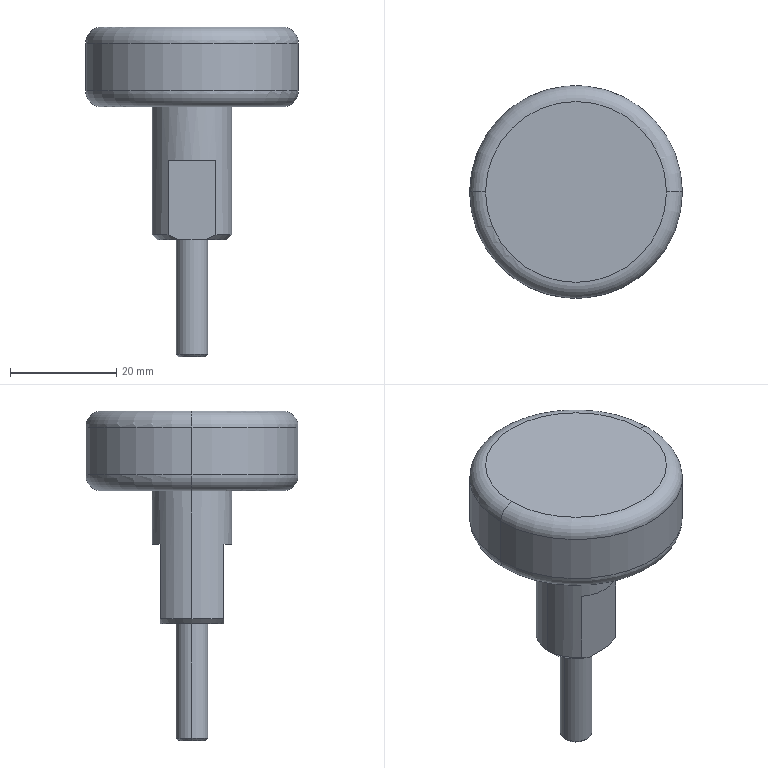Part | NX | features BREP 1 | 1 solid | 23 faces | box 40 x 40 x 62 mm | volume 23128 mm3 | plane 8 | cylinder 6 | cone 5 | torus 4 | commonest cylinder face diameters 6 x2 15 x2 40 x2
STEP:
#1=CARTESIAN_POINT('',(121.406,-247.447,47.));
#2=VERTEX_POINT('',#1);
#3=CARTESIAN_POINT('',(155.406,-247.447,47.));
#4=VERTEX_POINT('',#3);
#5=CARTESIAN_POINT('',(138.406,-247.447,47.));
#6=DIRECTION('',(0.,0.,-1.));
#7=DIRECTION('',(1.,0.,0.));
#8=AXIS2_PLACEMENT_3D('',#5,#6,#7);
#9=CIRCLE('',#8,17.);
#10=EDGE_CURVE('',#2,#4,#9,.T.);
#11=ORIENTED_EDGE('',*,*,#10,.F.);
#12=CARTESIAN_POINT('',(118.406,-247.447,50.));
#13=VERTEX_POINT('',#12);
#14=CARTESIAN_POINT('',(121.406,-247.447,50.));
#15=DIRECTION('',(0.,1.,0.));
#16=DIRECTION('',(-1.,0.,0.));
#17=AXIS2_PLACEMENT_3D('',#14,#15,#16);
#18=CIRCLE('',#17,3.);
#19=EDGE_CURVE('',#13,#2,#18,.F.);
#20=ORIENTED_EDGE('',*,*,#19,.F.);
#21=CARTESIAN_POINT('',(158.406,-247.447,50.));
#22=VERTEX_POINT('',#21);
#23=CARTESIAN_POINT('',(138.406,-247.447,50.));
#24=DIRECTION('',(0.,0.,1.));
#25=DIRECTION('',(1.,0.,0.));
#26=AXIS2_PLACEMENT_3D('',#23,#24,#25);
#27=CIRCLE('',#26,20.);
#28=EDGE_CURVE('',#22,#13,#27,.T.);
#29=ORIENTED_EDGE('',*,*,#28,.F.);
#30=CARTESIAN_POINT('',(155.406,-247.447,50.));
#31=DIRECTION('',(0.,-1.,0.));
#32=DIRECTION('',(0.,0.,-1.));
#33=AXIS2_PLACEMENT_3D('',#30,#31,#32);
#34=CIRCLE('',#33,3.);
#35=EDGE_CURVE('',#22,#4,#34,.F.);
#36=ORIENTED_EDGE('',*,*,#35,.T.);
#37=EDGE_LOOP('',(#11,#20,#29,#36));
#38=FACE_BOUND('',#37,.T.);
#39=CARTESIAN_POINT('',(138.406,-247.447,50.));
#40=DIRECTION('',(0.,0.,1.));
#41=DIRECTION('',(1.,0.,0.));
#42=AXIS2_PLACEMENT_3D('',#39,#40,#41);
#43=TOROIDAL_SURFACE('',#42,17.,3.);
#44=ADVANCED_FACE('',(#38),#43,.T.);
#45=CARTESIAN_POINT('',(118.406,-247.447,59.));
#46=VERTEX_POINT('',#45);
#47=CARTESIAN_POINT('',(158.406,-247.447,59.));
#48=VERTEX_POINT('',#47);
#49=CARTESIAN_POINT('',(138.406,-247.447,59.));
#50=DIRECTION('',(0.,0.,-1.));
#51=DIRECTION('',(1.,0.,0.));
#52=AXIS2_PLACEMENT_3D('',#49,#50,#51);
#53=CIRCLE('',#52,20.);
#54=EDGE_CURVE('',#46,#48,#53,.T.);
#55=ORIENTED_EDGE('',*,*,#54,.F.);
#56=CARTESIAN_POINT('',(121.406,-247.447,62.));
#57=VERTEX_POINT('',#56);
#58=CARTESIAN_POINT('',(121.406,-247.447,59.));
#59=DIRECTION('',(0.,1.,0.));
#60=DIRECTION('',(-1.,0.,0.));
#61=AXIS2_PLACEMENT_3D('',#58,#59,#60);
#62=CIRCLE('',#61,3.);
#63=EDGE_CURVE('',#57,#46,#62,.F.);
#64=ORIENTED_EDGE('',*,*,#63,.F.);
#65=CARTESIAN_POINT('',(155.406,-247.447,62.));
#66=VERTEX_POINT('',#65);
#67=CARTESIAN_POINT('',(138.406,-247.447,62.));
#68=DIRECTION('',(0.,0.,1.));
#69=DIRECTION('',(1.,0.,0.));
#70=AXIS2_PLACEMENT_3D('',#67,#68,#69);
#71=CIRCLE('',#70,17.);
#72=EDGE_CURVE('',#66,#57,#71,.T.);
#73=ORIENTED_EDGE('',*,*,#72,.F.);
#74=CARTESIAN_POINT('',(155.406,-247.447,59.));
#75=DIRECTION('',(0.,-1.,0.));
#76=DIRECTION('',(0.,0.,-1.));
#77=AXIS2_PLACEMENT_3D('',#74,#75,#76);
#78=CIRCLE('',#77,3.);
#79=EDGE_CURVE('',#66,#48,#78,.F.);
#80=ORIENTED_EDGE('',*,*,#79,.T.);
#81=EDGE_LOOP('',(#55,#64,#73,#80));
#82=FACE_BOUND('',#81,.T.);
#83=CARTESIAN_POINT('',(138.406,-247.447,59.));
#84=DIRECTION('',(0.,0.,1.));
#85=DIRECTION('',(1.,0.,0.));
#86=AXIS2_PLACEMENT_3D('',#83,#84,#85);
#87=TOROIDAL_SURFACE('',#86,17.,3.);
#88=ADVANCED_FACE('',(#82),#87,.T.);
#89=CARTESIAN_POINT('',(135.906,-247.447,0.));
#90=VERTEX_POINT('',#89);
#91=CARTESIAN_POINT('',(140.906,-247.447,0.));
#92=VERTEX_POINT('',#91);
#93=CARTESIAN_POINT('',(138.406,-247.447,0.));
#94=DIRECTION('',(0.,0.,-1.));
#95=DIRECTION('',(1.,0.,0.));
#96=AXIS2_PLACEMENT_3D('',#93,#94,#95);
#97=CIRCLE('',#96,2.5);
#98=EDGE_CURVE('',#90,#92,#97,.T.);
#99=ORIENTED_EDGE('',*,*,#98,.F.);
#100=CARTESIAN_POINT('',(135.406,-247.447,0.5));
#101=VERTEX_POINT('',#100);
#102=CARTESIAN_POINT('',(135.406,-247.447,0.5));
#103=DIRECTION('',(-0.7071,0.,0.7071));
#104=VECTOR('',#103,1000.);
#105=LINE('',#102,#104);
#106=EDGE_CURVE('',#101,#90,#105,.F.);
#107=ORIENTED_EDGE('',*,*,#106,.F.);
#108=CARTESIAN_POINT('',(141.406,-247.447,0.5));
#109=VERTEX_POINT('',#108);
#110=CARTESIAN_POINT('',(138.406,-247.447,0.5));
#111=DIRECTION('',(0.,0.,1.));
#112=DIRECTION('',(1.,0.,0.));
#113=AXIS2_PLACEMENT_3D('',#110,#111,#112);
#114=CIRCLE('',#113,3.);
#115=EDGE_CURVE('',#109,#101,#114,.T.);
#116=ORIENTED_EDGE('',*,*,#115,.F.);
#117=CARTESIAN_POINT('',(141.406,-247.447,0.5));
#118=DIRECTION('',(0.7071,0.,0.7071));
#119=VECTOR('',#118,1000.);
#120=LINE('',#117,#119);
#121=EDGE_CURVE('',#109,#92,#120,.F.);
#122=ORIENTED_EDGE('',*,*,#121,.T.);
#123=EDGE_LOOP('',(#99,#107,#116,#122));
#124=FACE_BOUND('',#123,.T.);
#125=CARTESIAN_POINT('',(138.406,-247.447,0.5));
#126=DIRECTION('',(0.,0.,1.));
#127=DIRECTION('',(1.,0.,0.));
#128=AXIS2_PLACEMENT_3D('',#125,#126,#127);
#129=CONICAL_SURFACE('',#128,3.,0.7854);
#130=ADVANCED_FACE('',(#124),#129,.T.);
#131=ORIENTED_EDGE('',*,*,#54,.T.);
#132=CARTESIAN_POINT('',(158.406,-247.447,62.));
#133=DIRECTION('',(0.,0.,-1.));
#134=VECTOR('',#133,1000.);
#135=LINE('',#132,#134);
#136=EDGE_CURVE('',#48,#22,#135,.T.);
#137=ORIENTED_EDGE('',*,*,#136,.T.);
#138=ORIENTED_EDGE('',*,*,#28,.T.);
#139=CARTESIAN_POINT('',(118.406,-247.447,62.));
#140=DIRECTION('',(0.,0.,-1.));
#141=VECTOR('',#140,1000.);
#142=LINE('',#139,#141);
#143=EDGE_CURVE('',#46,#13,#142,.T.);
#144=ORIENTED_EDGE('',*,*,#143,.F.);
#145=EDGE_LOOP('',(#131,#137,#138,#144));
#146=FACE_BOUND('',#145,.T.);
#147=CARTESIAN_POINT('',(138.406,-247.447,62.));
#148=DIRECTION('',(0.,0.,-1.));
#149=DIRECTION('',(-1.,0.,0.));
#150=AXIS2_PLACEMENT_3D('',#147,#148,#149);
#151=CYLINDRICAL_SURFACE('',#150,20.);
#152=ADVANCED_FACE('',(#146),#151,.T.);
#153=CARTESIAN_POINT('',(141.406,-247.447,22.));
#154=VERTEX_POINT('',#153);
#155=CARTESIAN_POINT('',(135.406,-247.447,22.));
#156=VERTEX_POINT('',#155);
#157=CARTESIAN_POINT('',(138.406,-247.447,22.));
#158=DIRECTION('',(0.,0.,1.));
#159=DIRECTION('',(1.,0.,0.));
#160=AXIS2_PLACEMENT_3D('',#157,#158,#159);
#161=CIRCLE('',#160,3.);
#162=EDGE_CURVE('',#154,#156,#161,.T.);
#163=ORIENTED_EDGE('',*,*,#162,.F.);
#164=CARTESIAN_POINT('',(141.406,-247.447,22.));
#165=DIRECTION('',(0.,0.,-1.));
#166=VECTOR('',#165,1000.);
#167=LINE('',#164,#166);
#168=EDGE_CURVE('',#154,#109,#167,.T.);
#169=ORIENTED_EDGE('',*,*,#168,.T.);
#170=ORIENTED_EDGE('',*,*,#115,.T.);
#171=CARTESIAN_POINT('',(135.406,-247.447,22.));
#172=DIRECTION('',(0.,0.,-1.));
#173=VECTOR('',#172,1000.);
#174=LINE('',#171,#173);
#175=EDGE_CURVE('',#156,#101,#174,.T.);
#176=ORIENTED_EDGE('',*,*,#175,.F.);
#177=EDGE_LOOP('',(#163,#169,#170,#176));
#178=FACE_BOUND('',#177,.T.);
#179=CARTESIAN_POINT('',(138.406,-247.447,22.));
#180=DIRECTION('',(0.,0.,-1.));
#181=DIRECTION('',(-1.,0.,0.));
#182=AXIS2_PLACEMENT_3D('',#179,#180,#181);
#183=CYLINDRICAL_SURFACE('',#182,3.);
#184=ADVANCED_FACE('',(#178),#183,.T.);
#185=CARTESIAN_POINT('',(144.906,-247.447,22.));
#186=VERTEX_POINT('',#185);
#187=CARTESIAN_POINT('',(140.906,-253.447,22.));
#188=VERTEX_POINT('',#187);
#189=CARTESIAN_POINT('',(138.406,-247.447,22.));
#190=DIRECTION('',(0.,0.,-1.));
#191=DIRECTION('',(1.,0.,0.));
#192=AXIS2_PLACEMENT_3D('',#189,#190,#191);
#193=CIRCLE('',#192,6.5);
#194=EDGE_CURVE('',#186,#188,#193,.T.);
#195=ORIENTED_EDGE('',*,*,#194,.F.);
#196=CARTESIAN_POINT('',(145.906,-247.447,23.));
#197=VERTEX_POINT('',#196);
#198=CARTESIAN_POINT('',(145.906,-247.447,23.));
#199=DIRECTION('',(0.7071,0.,0.7071));
#200=VECTOR('',#199,1000.);
#201=LINE('',#198,#200);
#202=EDGE_CURVE('',#186,#197,#201,.T.);
#203=ORIENTED_EDGE('',*,*,#202,.T.);
#204=CARTESIAN_POINT('',(142.906,-253.447,23.));
#205=VERTEX_POINT('',#204);
#206=CARTESIAN_POINT('',(138.406,-247.447,23.));
#207=DIRECTION('',(0.,0.,1.));
#208=DIRECTION('',(1.,0.,0.));
#209=AXIS2_PLACEMENT_3D('',#206,#207,#208);
#210=CIRCLE('',#209,7.5);
#211=EDGE_CURVE('',#205,#197,#210,.T.);
#212=ORIENTED_EDGE('',*,*,#211,.F.);
#213=CARTESIAN_POINT('',(140.906,-253.447,22.));
#214=CARTESIAN_POINT('',(141.539,-253.447,22.243));
#215=CARTESIAN_POINT('',(142.196,-253.447,22.574));
#216=CARTESIAN_POINT('',(142.906,-253.447,23.));
#217=B_SPLINE_CURVE_WITH_KNOTS('',3,(#213,#214,#215,#216),.UNSPECIFIED.,.F.,.F.,(4,4),(0.,1.),.UNSPECIFIED.);
#218=EDGE_CURVE('',#205,#188,#217,.F.);
#219=ORIENTED_EDGE('',*,*,#218,.T.);
#220=EDGE_LOOP('',(#195,#203,#212,#219));
#221=FACE_BOUND('',#220,.T.);
#222=CARTESIAN_POINT('',(138.406,-247.447,23.));
#223=DIRECTION('',(0.,0.,1.));
#224=DIRECTION('',(1.,0.,0.));
#225=AXIS2_PLACEMENT_3D('',#222,#223,#224);
#226=CONICAL_SURFACE('',#225,7.5,0.7854);
#227=ADVANCED_FACE('',(#221),#226,.T.);
#228=CARTESIAN_POINT('',(145.906,-247.447,47.));
#229=VERTEX_POINT('',#228);
#230=CARTESIAN_POINT('',(130.906,-247.447,47.));
#231=VERTEX_POINT('',#230);
#232=CARTESIAN_POINT('',(138.406,-247.447,47.));
#233=DIRECTION('',(0.,0.,1.));
#234=DIRECTION('',(1.,0.,0.));
#235=AXIS2_PLACEMENT_3D('',#232,#233,#234);
#236=CIRCLE('',#235,7.5);
#237=EDGE_CURVE('',#229,#231,#236,.T.);
#238=ORIENTED_EDGE('',*,*,#237,.F.);
#239=CARTESIAN_POINT('',(145.906,-247.447,47.));
#240=DIRECTION('',(0.,0.,-1.));
#241=VECTOR('',#240,1000.);
#242=LINE('',#239,#241);
#243=EDGE_CURVE('',#229,#197,#242,.T.);
#244=ORIENTED_EDGE('',*,*,#243,.T.);
#245=CARTESIAN_POINT('',(142.906,-241.447,23.));
#246=VERTEX_POINT('',#245);
#247=CARTESIAN_POINT('',(138.406,-247.447,23.));
#248=DIRECTION('',(0.,0.,1.));
#249=DIRECTION('',(1.,0.,0.));
#250=AXIS2_PLACEMENT_3D('',#247,#248,#249);
#251=CIRCLE('',#250,7.5);
#252=EDGE_CURVE('',#197,#246,#251,.T.);
#253=ORIENTED_EDGE('',*,*,#252,.T.);
#254=CARTESIAN_POINT('',(142.906,-241.447,37.));
#255=VERTEX_POINT('',#254);
#256=CARTESIAN_POINT('',(142.906,-241.447,47.));
#257=DIRECTION('',(0.,0.,-1.));
#258=VECTOR('',#257,1000.);
#259=LINE('',#256,#258);
#260=EDGE_CURVE('',#255,#246,#259,.T.);
#261=ORIENTED_EDGE('',*,*,#260,.F.);
#262=CARTESIAN_POINT('',(133.906,-241.447,37.));
#263=VERTEX_POINT('',#262);
#264=CARTESIAN_POINT('',(138.406,-247.447,37.));
#265=DIRECTION('',(0.,0.,-1.));
#266=DIRECTION('',(-1.,0.,0.));
#267=AXIS2_PLACEMENT_3D('',#264,#265,#266);
#268=CIRCLE('',#267,7.5);
#269=EDGE_CURVE('',#263,#255,#268,.T.);
#270=ORIENTED_EDGE('',*,*,#269,.F.);
#271=CARTESIAN_POINT('',(133.906,-241.447,23.));
#272=VERTEX_POINT('',#271);
#273=CARTESIAN_POINT('',(133.906,-241.447,47.));
#274=DIRECTION('',(0.,0.,1.));
#275=VECTOR('',#274,1000.);
#276=LINE('',#273,#275);
#277=EDGE_CURVE('',#272,#263,#276,.T.);
#278=ORIENTED_EDGE('',*,*,#277,.F.);
#279=CARTESIAN_POINT('',(130.906,-247.447,23.));
#280=VERTEX_POINT('',#279);
#281=CARTESIAN_POINT('',(138.406,-247.447,23.));
#282=DIRECTION('',(0.,0.,1.));
#283=DIRECTION('',(1.,0.,0.));
#284=AXIS2_PLACEMENT_3D('',#281,#282,#283);
#285=CIRCLE('',#284,7.5);
#286=EDGE_CURVE('',#272,#280,#285,.T.);
#287=ORIENTED_EDGE('',*,*,#286,.T.);
#288=CARTESIAN_POINT('',(130.906,-247.447,47.));
#289=DIRECTION('',(0.,0.,-1.));
#290=VECTOR('',#289,1000.);
#291=LINE('',#288,#290);
#292=EDGE_CURVE('',#231,#280,#291,.T.);
#293=ORIENTED_EDGE('',*,*,#292,.F.);
#294=EDGE_LOOP('',(#238,#244,#253,#261,#270,#278,#287,#293));
#295=FACE_BOUND('',#294,.T.);
#296=CARTESIAN_POINT('',(138.406,-247.447,47.));
#297=DIRECTION('',(0.,0.,-1.));
#298=DIRECTION('',(-1.,0.,0.));
#299=AXIS2_PLACEMENT_3D('',#296,#297,#298);
#300=CYLINDRICAL_SURFACE('',#299,7.5);
#301=ADVANCED_FACE('',(#295),#300,.T.);
#302=CARTESIAN_POINT('',(135.906,-253.447,22.));
#303=VERTEX_POINT('',#302);
#304=CARTESIAN_POINT('',(147.962,-253.447,22.));
#305=DIRECTION('',(-1.,0.,0.));
#306=VECTOR('',#305,1000.);
#307=LINE('',#304,#306);
#308=EDGE_CURVE('',#188,#303,#307,.T.);
#309=ORIENTED_EDGE('',*,*,#308,.T.);
#310=CARTESIAN_POINT('',(135.906,-241.447,22.));
#311=VERTEX_POINT('',#310);
#312=CARTESIAN_POINT('',(138.406,-247.447,22.));
#313=DIRECTION('',(0.,0.,-1.));
#314=DIRECTION('',(1.,0.,0.));
#315=AXIS2_PLACEMENT_3D('',#312,#313,#314);
#316=CIRCLE('',#315,6.5);
#317=EDGE_CURVE('',#303,#311,#316,.T.);
#318=ORIENTED_EDGE('',*,*,#317,.T.);
#319=CARTESIAN_POINT('',(140.906,-241.447,22.));
#320=VERTEX_POINT('',#319);
#321=CARTESIAN_POINT('',(147.962,-241.447,22.));
#322=DIRECTION('',(1.,0.,0.));
#323=VECTOR('',#322,1000.);
#324=LINE('',#321,#323);
#325=EDGE_CURVE('',#311,#320,#324,.T.);
#326=ORIENTED_EDGE('',*,*,#325,.T.);
#327=CARTESIAN_POINT('',(138.406,-247.447,22.));
#328=DIRECTION('',(0.,0.,-1.));
#329=DIRECTION('',(1.,0.,0.));
#330=AXIS2_PLACEMENT_3D('',#327,#328,#329);
#331=CIRCLE('',#330,6.5);
#332=EDGE_CURVE('',#320,#186,#331,.T.);
#333=ORIENTED_EDGE('',*,*,#332,.T.);
#334=ORIENTED_EDGE('',*,*,#194,.T.);
#335=EDGE_LOOP('',(#309,#318,#326,#333,#334));
#336=FACE_BOUND('',#335,.T.);
#337=CARTESIAN_POINT('',(138.406,-247.447,22.));
#338=DIRECTION('',(0.,0.,1.));
#339=DIRECTION('',(1.,0.,0.));
#340=AXIS2_PLACEMENT_3D('',#337,#338,#339);
#341=CIRCLE('',#340,3.);
#342=EDGE_CURVE('',#156,#154,#341,.T.);
#343=ORIENTED_EDGE('',*,*,#342,.T.);
#344=ORIENTED_EDGE('',*,*,#162,.T.);
#345=EDGE_LOOP('',(#343,#344));
#346=FACE_BOUND('',#345,.T.);
#347=CARTESIAN_POINT('',(138.406,-247.447,22.));
#348=DIRECTION('',(0.,0.,1.));
#349=DIRECTION('',(1.,0.,0.));
#350=AXIS2_PLACEMENT_3D('',#347,#348,#349);
#351=PLANE('',#350);
#352=ADVANCED_FACE('',(#336,#346),#351,.F.);
#353=ORIENTED_EDGE('',*,*,#243,.F.);
#354=CARTESIAN_POINT('',(138.406,-247.447,47.));
#355=DIRECTION('',(0.,0.,1.));
#356=DIRECTION('',(1.,0.,0.));
#357=AXIS2_PLACEMENT_3D('',#354,#355,#356);
#358=CIRCLE('',#357,7.5);
#359=EDGE_CURVE('',#231,#229,#358,.T.);
#360=ORIENTED_EDGE('',*,*,#359,.F.);
#361=ORIENTED_EDGE('',*,*,#292,.T.);
#362=CARTESIAN_POINT('',(133.906,-253.447,23.));
#363=VERTEX_POINT('',#362);
#364=CARTESIAN_POINT('',(138.406,-247.447,23.));
#365=DIRECTION('',(0.,0.,1.));
#366=DIRECTION('',(1.,0.,0.));
#367=AXIS2_PLACEMENT_3D('',#364,#365,#366);
#368=CIRCLE('',#367,7.5);
#369=EDGE_CURVE('',#280,#363,#368,.T.);
#370=ORIENTED_EDGE('',*,*,#369,.T.);
#371=CARTESIAN_POINT('',(133.906,-253.447,37.));
#372=VERTEX_POINT('',#371);
#373=CARTESIAN_POINT('',(133.906,-253.447,47.));
#374=DIRECTION('',(0.,0.,-1.));
#375=VECTOR('',#374,1000.);
#376=LINE('',#373,#375);
#377=EDGE_CURVE('',#372,#363,#376,.T.);
#378=ORIENTED_EDGE('',*,*,#377,.F.);
#379=CARTESIAN_POINT('',(142.906,-253.447,37.));
#380=VERTEX_POINT('',#379);
#381=CARTESIAN_POINT('',(138.406,-247.447,37.));
#382=DIRECTION('',(0.,0.,-1.));
#383=DIRECTION('',(-1.,0.,0.));
#384=AXIS2_PLACEMENT_3D('',#381,#382,#383);
#385=CIRCLE('',#384,7.5);
#386=EDGE_CURVE('',#380,#372,#385,.T.);
#387=ORIENTED_EDGE('',*,*,#386,.F.);
#388=CARTESIAN_POINT('',(142.906,-253.447,47.));
#389=DIRECTION('',(0.,0.,1.));
#390=VECTOR('',#389,1000.);
#391=LINE('',#388,#390);
#392=EDGE_CURVE('',#205,#380,#391,.T.);
#393=ORIENTED_EDGE('',*,*,#392,.F.);
#394=ORIENTED_EDGE('',*,*,#211,.T.);
#395=EDGE_LOOP('',(#353,#360,#361,#370,#378,#387,#393,#394));
#396=FACE_BOUND('',#395,.T.);
#397=CARTESIAN_POINT('',(138.406,-247.447,47.));
#398=DIRECTION('',(0.,0.,-1.));
#399=DIRECTION('',(-1.,0.,0.));
#400=AXIS2_PLACEMENT_3D('',#397,#398,#399);
#401=CYLINDRICAL_SURFACE('',#400,7.5);
#402=ADVANCED_FACE('',(#396),#401,.T.);
#403=ORIENTED_EDGE('',*,*,#202,.F.);
#404=ORIENTED_EDGE('',*,*,#332,.F.);
#405=CARTESIAN_POINT('',(142.906,-241.447,23.));
#406=CARTESIAN_POINT('',(142.196,-241.447,22.574));
#407=CARTESIAN_POINT('',(141.54,-241.447,22.244));
#408=CARTESIAN_POINT('',(140.906,-241.447,22.));
#409=B_SPLINE_CURVE_WITH_KNOTS('',3,(#405,#406,#407,#408),.UNSPECIFIED.,.F.,.F.,(4,4),(0.,1.),.UNSPECIFIED.);
#410=EDGE_CURVE('',#320,#246,#409,.F.);
#411=ORIENTED_EDGE('',*,*,#410,.T.);
#412=ORIENTED_EDGE('',*,*,#252,.F.);
#413=EDGE_LOOP('',(#403,#404,#411,#412));
#414=FACE_BOUND('',#413,.T.);
#415=CARTESIAN_POINT('',(138.406,-247.447,23.));
#416=DIRECTION('',(0.,0.,1.));
#417=DIRECTION('',(1.,0.,0.));
#418=AXIS2_PLACEMENT_3D('',#415,#416,#417);
#419=CONICAL_SURFACE('',#418,7.5,0.7854);
#420=ADVANCED_FACE('',(#414),#419,.T.);
#421=ORIENTED_EDGE('',*,*,#317,.F.);
#422=CARTESIAN_POINT('',(133.906,-253.447,23.));
#423=CARTESIAN_POINT('',(134.616,-253.447,22.574));
#424=CARTESIAN_POINT('',(135.272,-253.447,22.244));
#425=CARTESIAN_POINT('',(135.906,-253.447,22.));
#426=B_SPLINE_CURVE_WITH_KNOTS('',3,(#422,#423,#424,#425),.UNSPECIFIED.,.F.,.F.,(4,4),(0.,1.),.UNSPECIFIED.);
#427=EDGE_CURVE('',#303,#363,#426,.F.);
#428=ORIENTED_EDGE('',*,*,#427,.T.);
#429=ORIENTED_EDGE('',*,*,#369,.F.);
#430=ORIENTED_EDGE('',*,*,#286,.F.);
#431=CARTESIAN_POINT('',(135.906,-241.447,22.));
#432=CARTESIAN_POINT('',(135.273,-241.447,22.243));
#433=CARTESIAN_POINT('',(134.616,-241.447,22.574));
#434=CARTESIAN_POINT('',(133.906,-241.447,23.));
#435=B_SPLINE_CURVE_WITH_KNOTS('',3,(#431,#432,#433,#434),.UNSPECIFIED.,.F.,.F.,(4,4),(0.,1.),.UNSPECIFIED.);
#436=EDGE_CURVE('',#272,#311,#435,.F.);
#437=ORIENTED_EDGE('',*,*,#436,.T.);
#438=EDGE_LOOP('',(#421,#428,#429,#430,#437));
#439=FACE_BOUND('',#438,.T.);
#440=CARTESIAN_POINT('',(138.406,-247.447,23.));
#441=DIRECTION('',(0.,0.,1.));
#442=DIRECTION('',(1.,0.,0.));
#443=AXIS2_PLACEMENT_3D('',#440,#441,#442);
#444=CONICAL_SURFACE('',#443,7.5,0.7854);
#445=ADVANCED_FACE('',(#439),#444,.T.);
#446=ORIENTED_EDGE('',*,*,#168,.F.);
#447=ORIENTED_EDGE('',*,*,#342,.F.);
#448=ORIENTED_EDGE('',*,*,#175,.T.);
#449=CARTESIAN_POINT('',(138.406,-247.447,0.5));
#450=DIRECTION('',(0.,0.,1.));
#451=DIRECTION('',(1.,0.,0.));
#452=AXIS2_PLACEMENT_3D('',#449,#450,#451);
#453=CIRCLE('',#452,3.);
#454=EDGE_CURVE('',#101,#109,#453,.T.);
#455=ORIENTED_EDGE('',*,*,#454,.T.);
#456=EDGE_LOOP('',(#446,#447,#448,#455));
#457=FACE_BOUND('',#456,.T.);
#458=CARTESIAN_POINT('',(138.406,-247.447,22.));
#459=DIRECTION('',(0.,0.,-1.));
#460=DIRECTION('',(-1.,0.,0.));
#461=AXIS2_PLACEMENT_3D('',#458,#459,#460);
#462=CYLINDRICAL_SURFACE('',#461,3.);
#463=ADVANCED_FACE('',(#457),#462,.T.);
#464=CARTESIAN_POINT('',(138.406,-247.447,0.));
#465=DIRECTION('',(0.,0.,-1.));
#466=DIRECTION('',(1.,0.,0.));
#467=AXIS2_PLACEMENT_3D('',#464,#465,#466);
#468=CIRCLE('',#467,2.5);
#469=EDGE_CURVE('',#92,#90,#468,.T.);
#470=ORIENTED_EDGE('',*,*,#469,.T.);
#471=ORIENTED_EDGE('',*,*,#98,.T.);
#472=EDGE_LOOP('',(#470,#471));
#473=FACE_BOUND('',#472,.T.);
#474=CARTESIAN_POINT('',(138.406,-247.447,0.));
#475=DIRECTION('',(0.,0.,1.));
#476=DIRECTION('',(1.,0.,0.));
#477=AXIS2_PLACEMENT_3D('',#474,#475,#476);
#478=PLANE('',#477);
#479=ADVANCED_FACE('',(#473),#478,.F.);
#480=CARTESIAN_POINT('',(138.406,-247.447,47.));
#481=DIRECTION('',(0.,0.,-1.));
#482=DIRECTION('',(1.,0.,0.));
#483=AXIS2_PLACEMENT_3D('',#480,#481,#482);
#484=CIRCLE('',#483,17.);
#485=EDGE_CURVE('',#4,#2,#484,.T.);
#486=ORIENTED_EDGE('',*,*,#485,.T.);
#487=ORIENTED_EDGE('',*,*,#10,.T.);
#488=EDGE_LOOP('',(#486,#487));
#489=FACE_BOUND('',#488,.T.);
#490=ORIENTED_EDGE('',*,*,#359,.T.);
#491=ORIENTED_EDGE('',*,*,#237,.T.);
#492=EDGE_LOOP('',(#490,#491));
#493=FACE_BOUND('',#492,.T.);
#494=CARTESIAN_POINT('',(138.406,-247.447,47.));
#495=DIRECTION('',(0.,0.,1.));
#496=DIRECTION('',(1.,0.,0.));
#497=AXIS2_PLACEMENT_3D('',#494,#495,#496);
#498=PLANE('',#497);
#499=ADVANCED_FACE('',(#489,#493),#498,.F.);
#500=ORIENTED_EDGE('',*,*,#136,.F.);
#501=CARTESIAN_POINT('',(138.406,-247.447,59.));
#502=DIRECTION('',(0.,0.,-1.));
#503=DIRECTION('',(1.,0.,0.));
#504=AXIS2_PLACEMENT_3D('',#501,#502,#503);
#505=CIRCLE('',#504,20.);
#506=EDGE_CURVE('',#48,#46,#505,.T.);
#507=ORIENTED_EDGE('',*,*,#506,.T.);
#508=ORIENTED_EDGE('',*,*,#143,.T.);
#509=CARTESIAN_POINT('',(138.406,-247.447,50.));
#510=DIRECTION('',(0.,0.,1.));
#511=DIRECTION('',(1.,0.,0.));
#512=AXIS2_PLACEMENT_3D('',#509,#510,#511);
#513=CIRCLE('',#512,20.);
#514=EDGE_CURVE('',#13,#22,#513,.T.);
#515=ORIENTED_EDGE('',*,*,#514,.T.);
#516=EDGE_LOOP('',(#500,#507,#508,#515));
#517=FACE_BOUND('',#516,.T.);
#518=CARTESIAN_POINT('',(138.406,-247.447,62.));
#519=DIRECTION('',(0.,0.,-1.));
#520=DIRECTION('',(-1.,0.,0.));
#521=AXIS2_PLACEMENT_3D('',#518,#519,#520);
#522=CYLINDRICAL_SURFACE('',#521,20.);
#523=ADVANCED_FACE('',(#517),#522,.T.);
#524=ORIENTED_EDGE('',*,*,#72,.T.);
#525=CARTESIAN_POINT('',(138.406,-247.447,62.));
#526=DIRECTION('',(0.,0.,1.));
#527=DIRECTION('',(1.,0.,0.));
#528=AXIS2_PLACEMENT_3D('',#525,#526,#527);
#529=CIRCLE('',#528,17.);
#530=EDGE_CURVE('',#57,#66,#529,.T.);
#531=ORIENTED_EDGE('',*,*,#530,.T.);
#532=EDGE_LOOP('',(#524,#531));
#533=FACE_BOUND('',#532,.T.);
#534=CARTESIAN_POINT('',(138.406,-247.447,62.));
#535=DIRECTION('',(0.,0.,1.));
#536=DIRECTION('',(1.,0.,0.));
#537=AXIS2_PLACEMENT_3D('',#534,#535,#536);
#538=PLANE('',#537);
#539=ADVANCED_FACE('',(#533),#538,.T.);
#540=ORIENTED_EDGE('',*,*,#106,.T.);
#541=ORIENTED_EDGE('',*,*,#469,.F.);
#542=ORIENTED_EDGE('',*,*,#121,.F.);
#543=ORIENTED_EDGE('',*,*,#454,.F.);
#544=EDGE_LOOP('',(#540,#541,#542,#543));
#545=FACE_BOUND('',#544,.T.);
#546=CARTESIAN_POINT('',(138.406,-247.447,0.5));
#547=DIRECTION('',(0.,0.,1.));
#548=DIRECTION('',(1.,0.,0.));
#549=AXIS2_PLACEMENT_3D('',#546,#547,#548);
#550=CONICAL_SURFACE('',#549,3.,0.7854);
#551=ADVANCED_FACE('',(#545),#550,.T.);
#552=ORIENTED_EDGE('',*,*,#63,.T.);
#553=ORIENTED_EDGE('',*,*,#506,.F.);
#554=ORIENTED_EDGE('',*,*,#79,.F.);
#555=ORIENTED_EDGE('',*,*,#530,.F.);
#556=EDGE_LOOP('',(#552,#553,#554,#555));
#557=FACE_BOUND('',#556,.T.);
#558=CARTESIAN_POINT('',(138.406,-247.447,59.));
#559=DIRECTION('',(0.,0.,1.));
#560=DIRECTION('',(1.,0.,0.));
#561=AXIS2_PLACEMENT_3D('',#558,#559,#560);
#562=TOROIDAL_SURFACE('',#561,17.,3.);
#563=ADVANCED_FACE('',(#557),#562,.T.);
#564=ORIENTED_EDGE('',*,*,#19,.T.);
#565=ORIENTED_EDGE('',*,*,#485,.F.);
#566=ORIENTED_EDGE('',*,*,#35,.F.);
#567=ORIENTED_EDGE('',*,*,#514,.F.);
#568=EDGE_LOOP('',(#564,#565,#566,#567));
#569=FACE_BOUND('',#568,.T.);
#570=CARTESIAN_POINT('',(138.406,-247.447,50.));
#571=DIRECTION('',(0.,0.,1.));
#572=DIRECTION('',(1.,0.,0.));
#573=AXIS2_PLACEMENT_3D('',#570,#571,#572);
#574=TOROIDAL_SURFACE('',#573,17.,3.);
#575=ADVANCED_FACE('',(#569),#574,.T.);
#576=ORIENTED_EDGE('',*,*,#277,.T.);
#577=CARTESIAN_POINT('',(147.962,-241.447,37.));
#578=DIRECTION('',(1.,0.,0.));
#579=VECTOR('',#578,1000.);
#580=LINE('',#577,#579);
#581=EDGE_CURVE('',#263,#255,#580,.T.);
#582=ORIENTED_EDGE('',*,*,#581,.T.);
#583=ORIENTED_EDGE('',*,*,#260,.T.);
#584=ORIENTED_EDGE('',*,*,#410,.F.);
#585=ORIENTED_EDGE('',*,*,#325,.F.);
#586=ORIENTED_EDGE('',*,*,#436,.F.);
#587=EDGE_LOOP('',(#576,#582,#583,#584,#585,#586));
#588=FACE_BOUND('',#587,.T.);
#589=CARTESIAN_POINT('',(147.962,-241.447,37.));
#590=DIRECTION('',(0.,1.,0.));
#591=DIRECTION('',(1.,0.,0.));
#592=AXIS2_PLACEMENT_3D('',#589,#590,#591);
#593=PLANE('',#592);
#594=ADVANCED_FACE('',(#588),#593,.T.);
#595=ORIENTED_EDGE('',*,*,#269,.T.);
#596=ORIENTED_EDGE('',*,*,#581,.F.);
#597=EDGE_LOOP('',(#595,#596));
#598=FACE_BOUND('',#597,.T.);
#599=CARTESIAN_POINT('',(138.406,-247.447,37.));
#600=DIRECTION('',(0.,0.,-1.));
#601=DIRECTION('',(0.,-1.,0.));
#602=AXIS2_PLACEMENT_3D('',#599,#600,#601);
#603=PLANE('',#602);
#604=ADVANCED_FACE('',(#598),#603,.T.);
#605=ORIENTED_EDGE('',*,*,#386,.T.);
#606=CARTESIAN_POINT('',(147.962,-253.447,37.));
#607=DIRECTION('',(-1.,0.,0.));
#608=VECTOR('',#607,1000.);
#609=LINE('',#606,#608);
#610=EDGE_CURVE('',#380,#372,#609,.T.);
#611=ORIENTED_EDGE('',*,*,#610,.F.);
#612=EDGE_LOOP('',(#605,#611));
#613=FACE_BOUND('',#612,.T.);
#614=CARTESIAN_POINT('',(138.406,-247.447,37.));
#615=DIRECTION('',(0.,0.,-1.));
#616=DIRECTION('',(0.,-1.,0.));
#617=AXIS2_PLACEMENT_3D('',#614,#615,#616);
#618=PLANE('',#617);
#619=ADVANCED_FACE('',(#613),#618,.T.);
#620=ORIENTED_EDGE('',*,*,#392,.T.);
#621=ORIENTED_EDGE('',*,*,#610,.T.);
#622=ORIENTED_EDGE('',*,*,#377,.T.);
#623=ORIENTED_EDGE('',*,*,#427,.F.);
#624=ORIENTED_EDGE('',*,*,#308,.F.);
#625=ORIENTED_EDGE('',*,*,#218,.F.);
#626=EDGE_LOOP('',(#620,#621,#622,#623,#624,#625));
#627=FACE_BOUND('',#626,.T.);
#628=CARTESIAN_POINT('',(147.962,-253.447,37.));
#629=DIRECTION('',(0.,-1.,0.));
#630=DIRECTION('',(0.,0.,-1.));
#631=AXIS2_PLACEMENT_3D('',#628,#629,#630);
#632=PLANE('',#631);
#633=ADVANCED_FACE('',(#627),#632,.T.);
#634=CLOSED_SHELL('',(#44,#88,#130,#152,#184,#227,#301,#352,#402,#420,#445,#463,#479,#499,#523,#539,#551,#563,#575,#594,#604,#619,#633));
#635=MANIFOLD_SOLID_BREP('',#634);
#636=(LENGTH_UNIT()NAMED_UNIT(*)SI_UNIT(.MILLI.,.METRE.));
#637=UNCERTAINTY_MEASURE_WITH_UNIT(LENGTH_MEASURE(0.0508),#636,'','');
#638=(NAMED_UNIT(*)PLANE_ANGLE_UNIT()SI_UNIT($,.RADIAN.));
#639=(NAMED_UNIT(*)SI_UNIT($,.STERADIAN.)SOLID_ANGLE_UNIT());
#640=(GEOMETRIC_REPRESENTATION_CONTEXT(3)GLOBAL_UNCERTAINTY_ASSIGNED_CONTEXT((#637))GLOBAL_UNIT_ASSIGNED_CONTEXT((#636,#638,#639))REPRESENTATION_CONTEXT('',''));
#641=ADVANCED_BREP_SHAPE_REPRESENTATION('',(#635),#640);